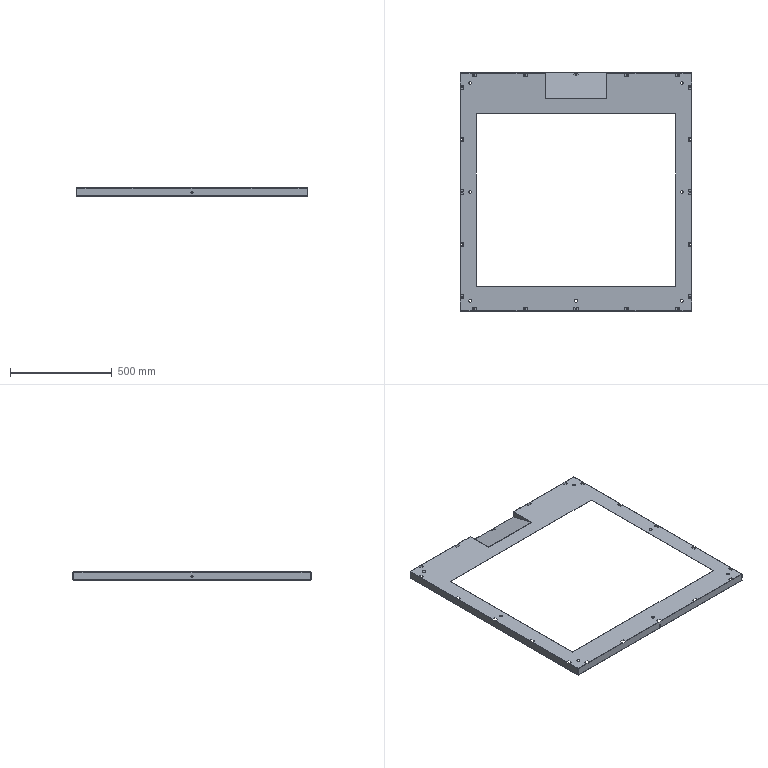Part | 2 solids | 408 faces | box 1139 x 1169 x 40 mm | volume 780725 mm3 | plane 258 | cylinder 130 | spline 20 | commonest cylinder face diameters 7 x50 0.4 x30 2.4 x30 14 x14 10 x6